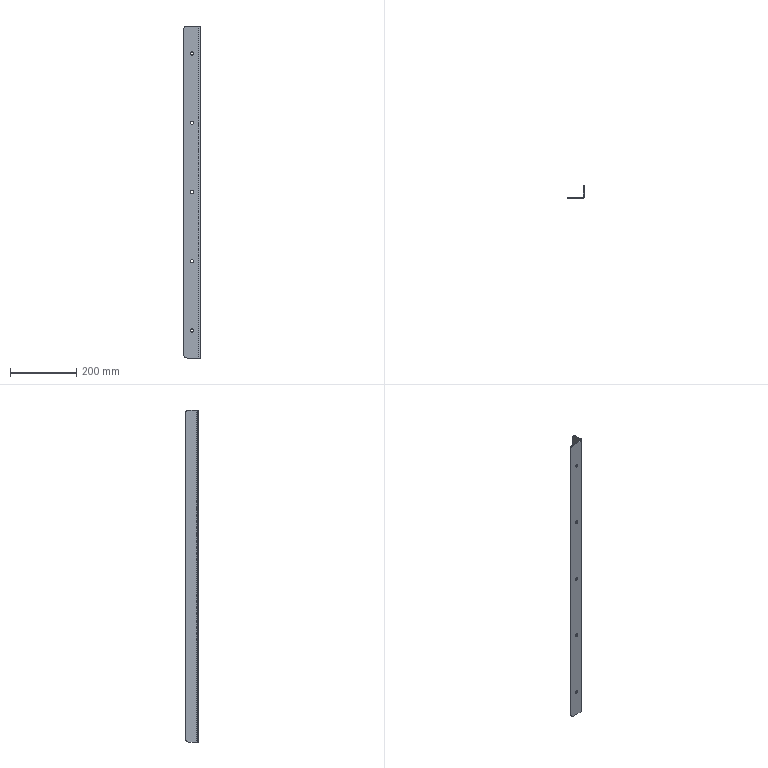Part | STEP file | 750078456 | 1 solid | 24 faces | box 50 x 40 x 1006 mm | volume 255301 mm3 | cylinder 16 | plane 8 | commonest cylinder face diameters 10 x10 20 x4 6 x1 12 x1
STEP:
#1=CARTESIAN_POINT('',(-20.,3.,210.));
#2=VERTEX_POINT('',#1);
#3=CARTESIAN_POINT('',(-30.,3.,210.));
#4=VERTEX_POINT('',#3);
#5=CARTESIAN_POINT('',(-25.,3.,210.));
#6=DIRECTION('',(0.,1.,0.));
#7=DIRECTION('',(1.,0.,0.));
#8=AXIS2_PLACEMENT_3D('',#5,#6,#7);
#9=CIRCLE('',#8,5.);
#10=EDGE_CURVE('',#2,#4,#9,.T.);
#11=ORIENTED_EDGE('',*,*,#10,.T.);
#12=CARTESIAN_POINT('',(-30.,0.,210.));
#13=VERTEX_POINT('',#12);
#14=CARTESIAN_POINT('',(-30.,1008.036,210.));
#15=DIRECTION('',(0.,-1.,0.));
#16=VECTOR('',#15,1000.);
#17=LINE('',#14,#16);
#18=EDGE_CURVE('',#4,#13,#17,.T.);
#19=ORIENTED_EDGE('',*,*,#18,.T.);
#20=CARTESIAN_POINT('',(-20.,0.,210.));
#21=VERTEX_POINT('',#20);
#22=CARTESIAN_POINT('',(-25.,0.,210.));
#23=DIRECTION('',(0.,1.,0.));
#24=DIRECTION('',(1.,0.,0.));
#25=AXIS2_PLACEMENT_3D('',#22,#23,#24);
#26=CIRCLE('',#25,5.);
#27=EDGE_CURVE('',#21,#13,#26,.T.);
#28=ORIENTED_EDGE('',*,*,#27,.F.);
#29=CARTESIAN_POINT('',(-20.,1008.036,210.));
#30=DIRECTION('',(0.,-1.,0.));
#31=VECTOR('',#30,1000.);
#32=LINE('',#29,#31);
#33=EDGE_CURVE('',#2,#21,#32,.T.);
#34=ORIENTED_EDGE('',*,*,#33,.F.);
#35=EDGE_LOOP('',(#11,#19,#28,#34));
#36=FACE_OUTER_BOUND('',#35,.T.);
#37=CARTESIAN_POINT('',(-25.,1008.036,210.));
#38=DIRECTION('',(0.,-1.,0.));
#39=DIRECTION('',(1.,0.,0.));
#40=AXIS2_PLACEMENT_3D('',#37,#38,#39);
#41=CYLINDRICAL_SURFACE('',#40,5.);
#42=ADVANCED_FACE('',(#36),#41,.F.);
#43=CARTESIAN_POINT('',(-20.,3.,-210.));
#44=VERTEX_POINT('',#43);
#45=CARTESIAN_POINT('',(-30.,3.,-210.));
#46=VERTEX_POINT('',#45);
#47=CARTESIAN_POINT('',(-25.,3.,-210.));
#48=DIRECTION('',(0.,1.,0.));
#49=DIRECTION('',(1.,0.,0.));
#50=AXIS2_PLACEMENT_3D('',#47,#48,#49);
#51=CIRCLE('',#50,5.);
#52=EDGE_CURVE('',#44,#46,#51,.T.);
#53=ORIENTED_EDGE('',*,*,#52,.T.);
#54=CARTESIAN_POINT('',(-30.,0.,-210.));
#55=VERTEX_POINT('',#54);
#56=CARTESIAN_POINT('',(-30.,1008.036,-210.));
#57=DIRECTION('',(0.,-1.,0.));
#58=VECTOR('',#57,1000.);
#59=LINE('',#56,#58);
#60=EDGE_CURVE('',#46,#55,#59,.T.);
#61=ORIENTED_EDGE('',*,*,#60,.T.);
#62=CARTESIAN_POINT('',(-20.,0.,-210.));
#63=VERTEX_POINT('',#62);
#64=CARTESIAN_POINT('',(-25.,0.,-210.));
#65=DIRECTION('',(0.,1.,0.));
#66=DIRECTION('',(1.,0.,0.));
#67=AXIS2_PLACEMENT_3D('',#64,#65,#66);
#68=CIRCLE('',#67,5.);
#69=EDGE_CURVE('',#63,#55,#68,.T.);
#70=ORIENTED_EDGE('',*,*,#69,.F.);
#71=CARTESIAN_POINT('',(-20.,1008.036,-210.));
#72=DIRECTION('',(0.,-1.,0.));
#73=VECTOR('',#72,1000.);
#74=LINE('',#71,#73);
#75=EDGE_CURVE('',#44,#63,#74,.T.);
#76=ORIENTED_EDGE('',*,*,#75,.F.);
#77=EDGE_LOOP('',(#53,#61,#70,#76));
#78=FACE_OUTER_BOUND('',#77,.T.);
#79=CARTESIAN_POINT('',(-25.,1008.036,-210.));
#80=DIRECTION('',(0.,-1.,0.));
#81=DIRECTION('',(1.,0.,0.));
#82=AXIS2_PLACEMENT_3D('',#79,#80,#81);
#83=CYLINDRICAL_SURFACE('',#82,5.);
#84=ADVANCED_FACE('',(#78),#83,.F.);
#85=CARTESIAN_POINT('',(-20.,3.,-420.));
#86=VERTEX_POINT('',#85);
#87=CARTESIAN_POINT('',(-30.,3.,-420.));
#88=VERTEX_POINT('',#87);
#89=CARTESIAN_POINT('',(-25.,3.,-420.));
#90=DIRECTION('',(0.,1.,0.));
#91=DIRECTION('',(1.,0.,0.));
#92=AXIS2_PLACEMENT_3D('',#89,#90,#91);
#93=CIRCLE('',#92,5.);
#94=EDGE_CURVE('',#86,#88,#93,.T.);
#95=ORIENTED_EDGE('',*,*,#94,.T.);
#96=CARTESIAN_POINT('',(-30.,0.,-420.));
#97=VERTEX_POINT('',#96);
#98=CARTESIAN_POINT('',(-30.,1008.036,-420.));
#99=DIRECTION('',(0.,-1.,0.));
#100=VECTOR('',#99,1000.);
#101=LINE('',#98,#100);
#102=EDGE_CURVE('',#88,#97,#101,.T.);
#103=ORIENTED_EDGE('',*,*,#102,.T.);
#104=CARTESIAN_POINT('',(-20.,0.,-420.));
#105=VERTEX_POINT('',#104);
#106=CARTESIAN_POINT('',(-25.,0.,-420.));
#107=DIRECTION('',(0.,1.,0.));
#108=DIRECTION('',(1.,0.,0.));
#109=AXIS2_PLACEMENT_3D('',#106,#107,#108);
#110=CIRCLE('',#109,5.);
#111=EDGE_CURVE('',#105,#97,#110,.T.);
#112=ORIENTED_EDGE('',*,*,#111,.F.);
#113=CARTESIAN_POINT('',(-20.,1008.036,-420.));
#114=DIRECTION('',(0.,-1.,0.));
#115=VECTOR('',#114,1000.);
#116=LINE('',#113,#115);
#117=EDGE_CURVE('',#86,#105,#116,.T.);
#118=ORIENTED_EDGE('',*,*,#117,.F.);
#119=EDGE_LOOP('',(#95,#103,#112,#118));
#120=FACE_OUTER_BOUND('',#119,.T.);
#121=CARTESIAN_POINT('',(-25.,1008.036,-420.));
#122=DIRECTION('',(0.,-1.,0.));
#123=DIRECTION('',(1.,0.,0.));
#124=AXIS2_PLACEMENT_3D('',#121,#122,#123);
#125=CYLINDRICAL_SURFACE('',#124,5.);
#126=ADVANCED_FACE('',(#120),#125,.F.);
#127=CARTESIAN_POINT('',(-20.,3.,0.));
#128=VERTEX_POINT('',#127);
#129=CARTESIAN_POINT('',(-30.,3.,0.));
#130=VERTEX_POINT('',#129);
#131=CARTESIAN_POINT('',(-25.,3.,0.));
#132=DIRECTION('',(0.,1.,0.));
#133=DIRECTION('',(1.,0.,0.));
#134=AXIS2_PLACEMENT_3D('',#131,#132,#133);
#135=CIRCLE('',#134,5.);
#136=EDGE_CURVE('',#128,#130,#135,.T.);
#137=ORIENTED_EDGE('',*,*,#136,.T.);
#138=CARTESIAN_POINT('',(-30.,0.,0.));
#139=VERTEX_POINT('',#138);
#140=CARTESIAN_POINT('',(-30.,1008.036,0.));
#141=DIRECTION('',(0.,-1.,0.));
#142=VECTOR('',#141,1000.);
#143=LINE('',#140,#142);
#144=EDGE_CURVE('',#130,#139,#143,.T.);
#145=ORIENTED_EDGE('',*,*,#144,.T.);
#146=CARTESIAN_POINT('',(-20.,0.,0.));
#147=VERTEX_POINT('',#146);
#148=CARTESIAN_POINT('',(-25.,0.,0.));
#149=DIRECTION('',(0.,1.,0.));
#150=DIRECTION('',(1.,0.,0.));
#151=AXIS2_PLACEMENT_3D('',#148,#149,#150);
#152=CIRCLE('',#151,5.);
#153=EDGE_CURVE('',#147,#139,#152,.T.);
#154=ORIENTED_EDGE('',*,*,#153,.F.);
#155=CARTESIAN_POINT('',(-20.,1008.036,0.));
#156=DIRECTION('',(0.,-1.,0.));
#157=VECTOR('',#156,1000.);
#158=LINE('',#155,#157);
#159=EDGE_CURVE('',#128,#147,#158,.T.);
#160=ORIENTED_EDGE('',*,*,#159,.F.);
#161=EDGE_LOOP('',(#137,#145,#154,#160));
#162=FACE_OUTER_BOUND('',#161,.T.);
#163=CARTESIAN_POINT('',(-25.,1008.036,0.));
#164=DIRECTION('',(0.,-1.,0.));
#165=DIRECTION('',(1.,0.,0.));
#166=AXIS2_PLACEMENT_3D('',#163,#164,#165);
#167=CYLINDRICAL_SURFACE('',#166,5.);
#168=ADVANCED_FACE('',(#162),#167,.F.);
#169=CARTESIAN_POINT('',(-20.,3.,420.));
#170=VERTEX_POINT('',#169);
#171=CARTESIAN_POINT('',(-30.,3.,420.));
#172=VERTEX_POINT('',#171);
#173=CARTESIAN_POINT('',(-25.,3.,420.));
#174=DIRECTION('',(0.,1.,0.));
#175=DIRECTION('',(1.,0.,0.));
#176=AXIS2_PLACEMENT_3D('',#173,#174,#175);
#177=CIRCLE('',#176,5.);
#178=EDGE_CURVE('',#170,#172,#177,.T.);
#179=ORIENTED_EDGE('',*,*,#178,.T.);
#180=CARTESIAN_POINT('',(-30.,0.,420.));
#181=VERTEX_POINT('',#180);
#182=CARTESIAN_POINT('',(-30.,1008.036,420.));
#183=DIRECTION('',(0.,-1.,0.));
#184=VECTOR('',#183,1000.);
#185=LINE('',#182,#184);
#186=EDGE_CURVE('',#172,#181,#185,.T.);
#187=ORIENTED_EDGE('',*,*,#186,.T.);
#188=CARTESIAN_POINT('',(-20.,0.,420.));
#189=VERTEX_POINT('',#188);
#190=CARTESIAN_POINT('',(-25.,0.,420.));
#191=DIRECTION('',(0.,1.,0.));
#192=DIRECTION('',(1.,0.,0.));
#193=AXIS2_PLACEMENT_3D('',#190,#191,#192);
#194=CIRCLE('',#193,5.);
#195=EDGE_CURVE('',#189,#181,#194,.T.);
#196=ORIENTED_EDGE('',*,*,#195,.F.);
#197=CARTESIAN_POINT('',(-20.,1008.036,420.));
#198=DIRECTION('',(0.,-1.,0.));
#199=VECTOR('',#198,1000.);
#200=LINE('',#197,#199);
#201=EDGE_CURVE('',#170,#189,#200,.T.);
#202=ORIENTED_EDGE('',*,*,#201,.F.);
#203=EDGE_LOOP('',(#179,#187,#196,#202));
#204=FACE_OUTER_BOUND('',#203,.T.);
#205=CARTESIAN_POINT('',(-25.,1008.036,420.));
#206=DIRECTION('',(0.,-1.,0.));
#207=DIRECTION('',(1.,0.,0.));
#208=AXIS2_PLACEMENT_3D('',#205,#206,#207);
#209=CYLINDRICAL_SURFACE('',#208,5.);
#210=ADVANCED_FACE('',(#204),#209,.F.);
#211=CARTESIAN_POINT('',(-40.,3.,503.));
#212=VERTEX_POINT('',#211);
#213=CARTESIAN_POINT('',(-50.,3.,493.));
#214=VERTEX_POINT('',#213);
#215=CARTESIAN_POINT('',(-40.,3.,493.));
#216=DIRECTION('',(0.,-1.,0.));
#217=DIRECTION('',(1.,0.,0.));
#218=AXIS2_PLACEMENT_3D('',#215,#216,#217);
#219=CIRCLE('',#218,10.);
#220=EDGE_CURVE('',#212,#214,#219,.T.);
#221=ORIENTED_EDGE('',*,*,#220,.F.);
#222=CARTESIAN_POINT('',(-6.,3.,503.));
#223=VERTEX_POINT('',#222);
#224=CARTESIAN_POINT('',(0.,3.,503.));
#225=DIRECTION('',(-1.,0.,0.));
#226=VECTOR('',#225,1000.);
#227=LINE('',#224,#226);
#228=EDGE_CURVE('',#223,#212,#227,.T.);
#229=ORIENTED_EDGE('',*,*,#228,.F.);
#230=CARTESIAN_POINT('',(-6.,3.,-503.));
#231=VERTEX_POINT('',#230);
#232=CARTESIAN_POINT('',(-6.,3.,503.));
#233=DIRECTION('',(0.,0.,1.));
#234=VECTOR('',#233,1000.);
#235=LINE('',#232,#234);
#236=EDGE_CURVE('',#231,#223,#235,.T.);
#237=ORIENTED_EDGE('',*,*,#236,.F.);
#238=CARTESIAN_POINT('',(-40.,3.,-503.));
#239=VERTEX_POINT('',#238);
#240=CARTESIAN_POINT('',(0.,3.,-503.));
#241=DIRECTION('',(1.,0.,0.));
#242=VECTOR('',#241,1000.);
#243=LINE('',#240,#242);
#244=EDGE_CURVE('',#239,#231,#243,.T.);
#245=ORIENTED_EDGE('',*,*,#244,.F.);
#246=CARTESIAN_POINT('',(-50.,3.,-493.));
#247=VERTEX_POINT('',#246);
#248=CARTESIAN_POINT('',(-40.,3.,-493.));
#249=DIRECTION('',(0.,-1.,0.));
#250=DIRECTION('',(-1.,0.,0.));
#251=AXIS2_PLACEMENT_3D('',#248,#249,#250);
#252=CIRCLE('',#251,10.);
#253=EDGE_CURVE('',#247,#239,#252,.T.);
#254=ORIENTED_EDGE('',*,*,#253,.F.);
#255=CARTESIAN_POINT('',(-50.,3.,503.));
#256=DIRECTION('',(0.,0.,-1.));
#257=VECTOR('',#256,1000.);
#258=LINE('',#255,#257);
#259=EDGE_CURVE('',#214,#247,#258,.T.);
#260=ORIENTED_EDGE('',*,*,#259,.F.);
#261=EDGE_LOOP('',(#221,#229,#237,#245,#254,#260));
#262=FACE_OUTER_BOUND('',#261,.T.);
#263=ORIENTED_EDGE('',*,*,#10,.F.);
#264=CARTESIAN_POINT('',(-25.,3.,210.));
#265=DIRECTION('',(0.,1.,0.));
#266=DIRECTION('',(1.,0.,0.));
#267=AXIS2_PLACEMENT_3D('',#264,#265,#266);
#268=CIRCLE('',#267,5.);
#269=EDGE_CURVE('',#4,#2,#268,.T.);
#270=ORIENTED_EDGE('',*,*,#269,.F.);
#271=EDGE_LOOP('',(#263,#270));
#272=FACE_BOUND('',#271,.T.);
#273=ORIENTED_EDGE('',*,*,#52,.F.);
#274=CARTESIAN_POINT('',(-25.,3.,-210.));
#275=DIRECTION('',(0.,1.,0.));
#276=DIRECTION('',(1.,0.,0.));
#277=AXIS2_PLACEMENT_3D('',#274,#275,#276);
#278=CIRCLE('',#277,5.);
#279=EDGE_CURVE('',#46,#44,#278,.T.);
#280=ORIENTED_EDGE('',*,*,#279,.F.);
#281=EDGE_LOOP('',(#273,#280));
#282=FACE_BOUND('',#281,.T.);
#283=ORIENTED_EDGE('',*,*,#94,.F.);
#284=CARTESIAN_POINT('',(-25.,3.,-420.));
#285=DIRECTION('',(0.,1.,0.));
#286=DIRECTION('',(1.,0.,0.));
#287=AXIS2_PLACEMENT_3D('',#284,#285,#286);
#288=CIRCLE('',#287,5.);
#289=EDGE_CURVE('',#88,#86,#288,.T.);
#290=ORIENTED_EDGE('',*,*,#289,.F.);
#291=EDGE_LOOP('',(#283,#290));
#292=FACE_BOUND('',#291,.T.);
#293=ORIENTED_EDGE('',*,*,#136,.F.);
#294=CARTESIAN_POINT('',(-25.,3.,0.));
#295=DIRECTION('',(0.,1.,0.));
#296=DIRECTION('',(1.,0.,0.));
#297=AXIS2_PLACEMENT_3D('',#294,#295,#296);
#298=CIRCLE('',#297,5.);
#299=EDGE_CURVE('',#130,#128,#298,.T.);
#300=ORIENTED_EDGE('',*,*,#299,.F.);
#301=EDGE_LOOP('',(#293,#300));
#302=FACE_BOUND('',#301,.T.);
#303=ORIENTED_EDGE('',*,*,#178,.F.);
#304=CARTESIAN_POINT('',(-25.,3.,420.));
#305=DIRECTION('',(0.,1.,0.));
#306=DIRECTION('',(1.,0.,0.));
#307=AXIS2_PLACEMENT_3D('',#304,#305,#306);
#308=CIRCLE('',#307,5.);
#309=EDGE_CURVE('',#172,#170,#308,.T.);
#310=ORIENTED_EDGE('',*,*,#309,.F.);
#311=EDGE_LOOP('',(#303,#310));
#312=FACE_BOUND('',#311,.T.);
#313=CARTESIAN_POINT('',(0.,3.,503.));
#314=DIRECTION('',(0.,-1.,0.));
#315=DIRECTION('',(1.,0.,0.));
#316=AXIS2_PLACEMENT_3D('',#313,#314,#315);
#317=PLANE('',#316);
#318=ADVANCED_FACE('',(#262,#272,#282,#292,#302,#312),#317,.F.);
#319=ORIENTED_EDGE('',*,*,#259,.T.);
#320=CARTESIAN_POINT('',(-50.,0.,-493.));
#321=VERTEX_POINT('',#320);
#322=CARTESIAN_POINT('',(-50.,0.,-493.));
#323=DIRECTION('',(0.,-1.,0.));
#324=VECTOR('',#323,1000.);
#325=LINE('',#322,#324);
#326=EDGE_CURVE('',#247,#321,#325,.T.);
#327=ORIENTED_EDGE('',*,*,#326,.T.);
#328=CARTESIAN_POINT('',(-50.,0.,493.));
#329=VERTEX_POINT('',#328);
#330=CARTESIAN_POINT('',(-50.,0.,503.));
#331=DIRECTION('',(0.,0.,1.));
#332=VECTOR('',#331,1000.);
#333=LINE('',#330,#332);
#334=EDGE_CURVE('',#321,#329,#333,.T.);
#335=ORIENTED_EDGE('',*,*,#334,.T.);
#336=CARTESIAN_POINT('',(-50.,0.,493.));
#337=DIRECTION('',(0.,1.,0.));
#338=VECTOR('',#337,1000.);
#339=LINE('',#336,#338);
#340=EDGE_CURVE('',#329,#214,#339,.T.);
#341=ORIENTED_EDGE('',*,*,#340,.T.);
#342=EDGE_LOOP('',(#319,#327,#335,#341));
#343=FACE_OUTER_BOUND('',#342,.T.);
#344=CARTESIAN_POINT('',(-50.,0.,503.));
#345=DIRECTION('',(-1.,0.,0.));
#346=DIRECTION('',(0.,-1.,0.));
#347=AXIS2_PLACEMENT_3D('',#344,#345,#346);
#348=PLANE('',#347);
#349=ADVANCED_FACE('',(#343),#348,.T.);
#350=CARTESIAN_POINT('',(-40.,0.,503.));
#351=VERTEX_POINT('',#350);
#352=CARTESIAN_POINT('',(-40.,0.,493.));
#353=DIRECTION('',(0.,1.,0.));
#354=DIRECTION('',(1.,0.,0.));
#355=AXIS2_PLACEMENT_3D('',#352,#353,#354);
#356=CIRCLE('',#355,10.);
#357=EDGE_CURVE('',#329,#351,#356,.T.);
#358=ORIENTED_EDGE('',*,*,#357,.T.);
#359=CARTESIAN_POINT('',(-40.,0.,503.));
#360=DIRECTION('',(0.,1.,0.));
#361=VECTOR('',#360,1000.);
#362=LINE('',#359,#361);
#363=EDGE_CURVE('',#351,#212,#362,.T.);
#364=ORIENTED_EDGE('',*,*,#363,.T.);
#365=ORIENTED_EDGE('',*,*,#220,.T.);
#366=ORIENTED_EDGE('',*,*,#340,.F.);
#367=EDGE_LOOP('',(#358,#364,#365,#366));
#368=FACE_OUTER_BOUND('',#367,.T.);
#369=CARTESIAN_POINT('',(-40.,0.,493.));
#370=DIRECTION('',(0.,-1.,0.));
#371=DIRECTION('',(1.,0.,0.));
#372=AXIS2_PLACEMENT_3D('',#369,#370,#371);
#373=CYLINDRICAL_SURFACE('',#372,10.);
#374=ADVANCED_FACE('',(#368),#373,.T.);
#375=CARTESIAN_POINT('',(-6.,0.,503.));
#376=VERTEX_POINT('',#375);
#377=CARTESIAN_POINT('',(0.,0.,503.));
#378=DIRECTION('',(1.,0.,0.));
#379=VECTOR('',#378,1000.);
#380=LINE('',#377,#379);
#381=EDGE_CURVE('',#351,#376,#380,.T.);
#382=ORIENTED_EDGE('',*,*,#381,.T.);
#383=CARTESIAN_POINT('',(0.,6.,503.));
#384=VERTEX_POINT('',#383);
#385=CARTESIAN_POINT('',(-6.,6.,503.));
#386=DIRECTION('',(0.,0.,1.));
#387=DIRECTION('',(-1.,0.,0.));
#388=AXIS2_PLACEMENT_3D('',#385,#386,#387);
#389=CIRCLE('',#388,6.);
#390=EDGE_CURVE('',#376,#384,#389,.T.);
#391=ORIENTED_EDGE('',*,*,#390,.T.);
#392=CARTESIAN_POINT('',(0.,30.,503.));
#393=VERTEX_POINT('',#392);
#394=CARTESIAN_POINT('',(0.,0.,503.));
#395=DIRECTION('',(0.,1.,0.));
#396=VECTOR('',#395,1000.);
#397=LINE('',#394,#396);
#398=EDGE_CURVE('',#384,#393,#397,.T.);
#399=ORIENTED_EDGE('',*,*,#398,.T.);
#400=CARTESIAN_POINT('',(-3.,30.,503.));
#401=VERTEX_POINT('',#400);
#402=CARTESIAN_POINT('',(0.,30.,503.));
#403=DIRECTION('',(-1.,0.,0.));
#404=VECTOR('',#403,1000.);
#405=LINE('',#402,#404);
#406=EDGE_CURVE('',#393,#401,#405,.T.);
#407=ORIENTED_EDGE('',*,*,#406,.T.);
#408=CARTESIAN_POINT('',(-3.,6.,503.));
#409=VERTEX_POINT('',#408);
#410=CARTESIAN_POINT('',(-3.,0.,503.));
#411=DIRECTION('',(0.,-1.,0.));
#412=VECTOR('',#411,1000.);
#413=LINE('',#410,#412);
#414=EDGE_CURVE('',#401,#409,#413,.T.);
#415=ORIENTED_EDGE('',*,*,#414,.T.);
#416=CARTESIAN_POINT('',(-6.,6.,503.));
#417=DIRECTION('',(0.,0.,-1.));
#418=DIRECTION('',(-1.,0.,0.));
#419=AXIS2_PLACEMENT_3D('',#416,#417,#418);
#420=CIRCLE('',#419,3.);
#421=EDGE_CURVE('',#409,#223,#420,.T.);
#422=ORIENTED_EDGE('',*,*,#421,.T.);
#423=ORIENTED_EDGE('',*,*,#228,.T.);
#424=ORIENTED_EDGE('',*,*,#363,.F.);
#425=EDGE_LOOP('',(#382,#391,#399,#407,#415,#422,#423,#424));
#426=FACE_OUTER_BOUND('',#425,.T.);
#427=CARTESIAN_POINT('',(0.,0.,503.));
#428=DIRECTION('',(0.,0.,1.));
#429=DIRECTION('',(1.,0.,0.));
#430=AXIS2_PLACEMENT_3D('',#427,#428,#429);
#431=PLANE('',#430);
#432=ADVANCED_FACE('',(#426),#431,.T.);
#433=ORIENTED_EDGE('',*,*,#236,.T.);
#434=ORIENTED_EDGE('',*,*,#421,.F.);
#435=CARTESIAN_POINT('',(-3.,6.,-503.));
#436=VERTEX_POINT('',#435);
#437=CARTESIAN_POINT('',(-3.,6.,503.));
#438=DIRECTION('',(0.,0.,1.));
#439=VECTOR('',#438,1000.);
#440=LINE('',#437,#439);
#441=EDGE_CURVE('',#436,#409,#440,.T.);
#442=ORIENTED_EDGE('',*,*,#441,.F.);
#443=CARTESIAN_POINT('',(-6.,6.,-503.));
#444=DIRECTION('',(0.,0.,1.));
#445=DIRECTION('',(-1.,0.,0.));
#446=AXIS2_PLACEMENT_3D('',#443,#444,#445);
#447=CIRCLE('',#446,3.);
#448=EDGE_CURVE('',#231,#436,#447,.T.);
#449=ORIENTED_EDGE('',*,*,#448,.F.);
#450=EDGE_LOOP('',(#433,#434,#442,#449));
#451=FACE_OUTER_BOUND('',#450,.T.);
#452=CARTESIAN_POINT('',(-6.,6.,503.));
#453=DIRECTION('',(0.,0.,-1.));
#454=DIRECTION('',(-1.,0.,0.));
#455=AXIS2_PLACEMENT_3D('',#452,#453,#454);
#456=CYLINDRICAL_SURFACE('',#455,3.);
#457=ADVANCED_FACE('',(#451),#456,.F.);
#458=CARTESIAN_POINT('',(-40.,0.,-503.));
#459=VERTEX_POINT('',#458);
#460=CARTESIAN_POINT('',(-40.,40.,-503.));
#461=DIRECTION('',(0.,-1.,0.));
#462=VECTOR('',#461,1000.);
#463=LINE('',#460,#462);
#464=EDGE_CURVE('',#239,#459,#463,.T.);
#465=ORIENTED_EDGE('',*,*,#464,.F.);
#466=ORIENTED_EDGE('',*,*,#244,.T.);
#467=ORIENTED_EDGE('',*,*,#448,.T.);
#468=CARTESIAN_POINT('',(-3.,30.,-503.));
#469=VERTEX_POINT('',#468);
#470=CARTESIAN_POINT('',(-3.,40.,-503.));
#471=DIRECTION('',(0.,-1.,0.));
#472=VECTOR('',#471,1000.);
#473=LINE('',#470,#472);
#474=EDGE_CURVE('',#469,#436,#473,.T.);
#475=ORIENTED_EDGE('',*,*,#474,.F.);
#476=CARTESIAN_POINT('',(0.,30.,-503.));
#477=VERTEX_POINT('',#476);
#478=CARTESIAN_POINT('',(0.,30.,-503.));
#479=DIRECTION('',(-1.,0.,0.));
#480=VECTOR('',#479,1000.);
#481=LINE('',#478,#480);
#482=EDGE_CURVE('',#477,#469,#481,.T.);
#483=ORIENTED_EDGE('',*,*,#482,.F.);
#484=CARTESIAN_POINT('',(0.,6.,-503.));
#485=VERTEX_POINT('',#484);
#486=CARTESIAN_POINT('',(0.,40.,-503.));
#487=DIRECTION('',(0.,1.,0.));
#488=VECTOR('',#487,1000.);
#489=LINE('',#486,#488);
#490=EDGE_CURVE('',#485,#477,#489,.T.);
#491=ORIENTED_EDGE('',*,*,#490,.F.);
#492=CARTESIAN_POINT('',(-6.,0.,-503.));
#493=VERTEX_POINT('',#492);
#494=CARTESIAN_POINT('',(-6.,6.,-503.));
#495=DIRECTION('',(0.,0.,1.));
#496=DIRECTION('',(-1.,0.,0.));
#497=AXIS2_PLACEMENT_3D('',#494,#495,#496);
#498=CIRCLE('',#497,6.);
#499=EDGE_CURVE('',#493,#485,#498,.T.);
#500=ORIENTED_EDGE('',*,*,#499,.F.);
#501=CARTESIAN_POINT('',(0.,0.,-503.));
#502=DIRECTION('',(1.,0.,0.));
#503=VECTOR('',#502,1000.);
#504=LINE('',#501,#503);
#505=EDGE_CURVE('',#459,#493,#504,.T.);
#506=ORIENTED_EDGE('',*,*,#505,.F.);
#507=EDGE_LOOP('',(#465,#466,#467,#475,#483,#491,#500,#506));
#508=FACE_OUTER_BOUND('',#507,.T.);
#509=CARTESIAN_POINT('',(0.,40.,-503.));
#510=DIRECTION('',(0.,0.,1.));
#511=DIRECTION('',(1.,0.,0.));
#512=AXIS2_PLACEMENT_3D('',#509,#510,#511);
#513=PLANE('',#512);
#514=ADVANCED_FACE('',(#508),#513,.F.);
#515=CARTESIAN_POINT('',(-40.,0.,-493.));
#516=DIRECTION('',(0.,1.,0.));
#517=DIRECTION('',(-1.,0.,0.));
#518=AXIS2_PLACEMENT_3D('',#515,#516,#517);
#519=CIRCLE('',#518,10.);
#520=EDGE_CURVE('',#459,#321,#519,.T.);
#521=ORIENTED_EDGE('',*,*,#520,.T.);
#522=ORIENTED_EDGE('',*,*,#326,.F.);
#523=ORIENTED_EDGE('',*,*,#253,.T.);
#524=ORIENTED_EDGE('',*,*,#464,.T.);
#525=EDGE_LOOP('',(#521,#522,#523,#524));
#526=FACE_OUTER_BOUND('',#525,.T.);
#527=CARTESIAN_POINT('',(-40.,0.,-493.));
#528=DIRECTION('',(0.,1.,0.));
#529=DIRECTION('',(-1.,0.,0.));
#530=AXIS2_PLACEMENT_3D('',#527,#528,#529);
#531=CYLINDRICAL_SURFACE('',#530,10.);
#532=ADVANCED_FACE('',(#526),#531,.T.);
#533=ORIENTED_EDGE('',*,*,#18,.F.);
#534=ORIENTED_EDGE('',*,*,#269,.T.);
#535=ORIENTED_EDGE('',*,*,#33,.T.);
#536=CARTESIAN_POINT('',(-25.,0.,210.));
#537=DIRECTION('',(0.,1.,0.));
#538=DIRECTION('',(1.,0.,0.));
#539=AXIS2_PLACEMENT_3D('',#536,#537,#538);
#540=CIRCLE('',#539,5.);
#541=EDGE_CURVE('',#13,#21,#540,.T.);
#542=ORIENTED_EDGE('',*,*,#541,.F.);
#543=EDGE_LOOP('',(#533,#534,#535,#542));
#544=FACE_OUTER_BOUND('',#543,.T.);
#545=CARTESIAN_POINT('',(-25.,1008.036,210.));
#546=DIRECTION('',(0.,-1.,0.));
#547=DIRECTION('',(1.,0.,0.));
#548=AXIS2_PLACEMENT_3D('',#545,#546,#547);
#549=CYLINDRICAL_SURFACE('',#548,5.);
#550=ADVANCED_FACE('',(#544),#549,.F.);
#551=ORIENTED_EDGE('',*,*,#60,.F.);
#552=ORIENTED_EDGE('',*,*,#279,.T.);
#553=ORIENTED_EDGE('',*,*,#75,.T.);
#554=CARTESIAN_POINT('',(-25.,0.,-210.));
#555=DIRECTION('',(0.,1.,0.));
#556=DIRECTION('',(1.,0.,0.));
#557=AXIS2_PLACEMENT_3D('',#554,#555,#556);
#558=CIRCLE('',#557,5.);
#559=EDGE_CURVE('',#55,#63,#558,.T.);
#560=ORIENTED_EDGE('',*,*,#559,.F.);
#561=EDGE_LOOP('',(#551,#552,#553,#560));
#562=FACE_OUTER_BOUND('',#561,.T.);
#563=CARTESIAN_POINT('',(-25.,1008.036,-210.));
#564=DIRECTION('',(0.,-1.,0.));
#565=DIRECTION('',(1.,0.,0.));
#566=AXIS2_PLACEMENT_3D('',#563,#564,#565);
#567=CYLINDRICAL_SURFACE('',#566,5.);
#568=ADVANCED_FACE('',(#562),#567,.F.);
#569=ORIENTED_EDGE('',*,*,#102,.F.);
#570=ORIENTED_EDGE('',*,*,#289,.T.);
#571=ORIENTED_EDGE('',*,*,#117,.T.);
#572=CARTESIAN_POINT('',(-25.,0.,-420.));
#573=DIRECTION('',(0.,1.,0.));
#574=DIRECTION('',(1.,0.,0.));
#575=AXIS2_PLACEMENT_3D('',#572,#573,#574);
#576=CIRCLE('',#575,5.);
#577=EDGE_CURVE('',#97,#105,#576,.T.);
#578=ORIENTED_EDGE('',*,*,#577,.F.);
#579=EDGE_LOOP('',(#569,#570,#571,#578));
#580=FACE_OUTER_BOUND('',#579,.T.);
#581=CARTESIAN_POINT('',(-25.,1008.036,-420.));
#582=DIRECTION('',(0.,-1.,0.));
#583=DIRECTION('',(1.,0.,0.));
#584=AXIS2_PLACEMENT_3D('',#581,#582,#583);
#585=CYLINDRICAL_SURFACE('',#584,5.);
#586=ADVANCED_FACE('',(#580),#585,.F.);
#587=ORIENTED_EDGE('',*,*,#144,.F.);
#588=ORIENTED_EDGE('',*,*,#299,.T.);
#589=ORIENTED_EDGE('',*,*,#159,.T.);
#590=CARTESIAN_POINT('',(-25.,0.,0.));
#591=DIRECTION('',(0.,1.,0.));
#592=DIRECTION('',(1.,0.,0.));
#593=AXIS2_PLACEMENT_3D('',#590,#591,#592);
#594=CIRCLE('',#593,5.);
#595=EDGE_CURVE('',#139,#147,#594,.T.);
#596=ORIENTED_EDGE('',*,*,#595,.F.);
#597=EDGE_LOOP('',(#587,#588,#589,#596));
#598=FACE_OUTER_BOUND('',#597,.T.);
#599=CARTESIAN_POINT('',(-25.,1008.036,0.));
#600=DIRECTION('',(0.,-1.,0.));
#601=DIRECTION('',(1.,0.,0.));
#602=AXIS2_PLACEMENT_3D('',#599,#600,#601);
#603=CYLINDRICAL_SURFACE('',#602,5.);
#604=ADVANCED_FACE('',(#598),#603,.F.);
#605=ORIENTED_EDGE('',*,*,#186,.F.);
#606=ORIENTED_EDGE('',*,*,#309,.T.);
#607=ORIENTED_EDGE('',*,*,#201,.T.);
#608=CARTESIAN_POINT('',(-25.,0.,420.));
#609=DIRECTION('',(0.,1.,0.));
#610=DIRECTION('',(1.,0.,0.));
#611=AXIS2_PLACEMENT_3D('',#608,#609,#610);
#612=CIRCLE('',#611,5.);
#613=EDGE_CURVE('',#181,#189,#612,.T.);
#614=ORIENTED_EDGE('',*,*,#613,.F.);
#615=EDGE_LOOP('',(#605,#606,#607,#614));
#616=FACE_OUTER_BOUND('',#615,.T.);
#617=CARTESIAN_POINT('',(-25.,1008.036,420.));
#618=DIRECTION('',(0.,-1.,0.));
#619=DIRECTION('',(1.,0.,0.));
#620=AXIS2_PLACEMENT_3D('',#617,#618,#619);
#621=CYLINDRICAL_SURFACE('',#620,5.);
#622=ADVANCED_FACE('',(#616),#621,.F.);
#623=ORIENTED_EDGE('',*,*,#505,.T.);
#624=CARTESIAN_POINT('',(-6.,0.,503.));
#625=DIRECTION('',(0.,0.,1.));
#626=VECTOR('',#625,1000.);
#627=LINE('',#624,#626);
#628=EDGE_CURVE('',#493,#376,#627,.T.);
#629=ORIENTED_EDGE('',*,*,#628,.T.);
#630=ORIENTED_EDGE('',*,*,#381,.F.);
#631=ORIENTED_EDGE('',*,*,#357,.F.);
#632=ORIENTED_EDGE('',*,*,#334,.F.);
#633=ORIENTED_EDGE('',*,*,#520,.F.);
#634=EDGE_LOOP('',(#623,#629,#630,#631,#632,#633));
#635=FACE_OUTER_BOUND('',#634,.T.);
#636=ORIENTED_EDGE('',*,*,#27,.T.);
#637=ORIENTED_EDGE('',*,*,#541,.T.);
#638=EDGE_LOOP('',(#636,#637));
#639=FACE_BOUND('',#638,.T.);
#640=ORIENTED_EDGE('',*,*,#69,.T.);
#641=ORIENTED_EDGE('',*,*,#559,.T.);
#642=EDGE_LOOP('',(#640,#641));
#643=FACE_BOUND('',#642,.T.);
#644=ORIENTED_EDGE('',*,*,#111,.T.);
#645=ORIENTED_EDGE('',*,*,#577,.T.);
#646=EDGE_LOOP('',(#644,#645));
#647=FACE_BOUND('',#646,.T.);
#648=ORIENTED_EDGE('',*,*,#153,.T.);
#649=ORIENTED_EDGE('',*,*,#595,.T.);
#650=EDGE_LOOP('',(#648,#649));
#651=FACE_BOUND('',#650,.T.);
#652=ORIENTED_EDGE('',*,*,#195,.T.);
#653=ORIENTED_EDGE('',*,*,#613,.T.);
#654=EDGE_LOOP('',(#652,#653));
#655=FACE_BOUND('',#654,.T.);
#656=CARTESIAN_POINT('',(0.,0.,503.));
#657=DIRECTION('',(0.,-1.,0.));
#658=DIRECTION('',(1.,0.,0.));
#659=AXIS2_PLACEMENT_3D('',#656,#657,#658);
#660=PLANE('',#659);
#661=ADVANCED_FACE('',(#635,#639,#643,#647,#651,#655),#660,.T.);
#662=ORIENTED_EDGE('',*,*,#390,.F.);
#663=ORIENTED_EDGE('',*,*,#628,.F.);
#664=ORIENTED_EDGE('',*,*,#499,.T.);
#665=CARTESIAN_POINT('',(0.,6.,503.));
#666=DIRECTION('',(0.,0.,1.));
#667=VECTOR('',#666,1000.);
#668=LINE('',#665,#667);
#669=EDGE_CURVE('',#485,#384,#668,.T.);
#670=ORIENTED_EDGE('',*,*,#669,.T.);
#671=EDGE_LOOP('',(#662,#663,#664,#670));
#672=FACE_OUTER_BOUND('',#671,.T.);
#673=CARTESIAN_POINT('',(-6.,6.,503.));
#674=DIRECTION('',(0.,0.,-1.));
#675=DIRECTION('',(-1.,0.,0.));
#676=AXIS2_PLACEMENT_3D('',#673,#674,#675);
#677=CYLINDRICAL_SURFACE('',#676,6.);
#678=ADVANCED_FACE('',(#672),#677,.T.);
#679=CARTESIAN_POINT('',(-3.,40.,493.));
#680=VERTEX_POINT('',#679);
#681=CARTESIAN_POINT('',(-3.,30.,493.));
#682=DIRECTION('',(1.,0.,0.));
#683=DIRECTION('',(0.,0.,1.));
#684=AXIS2_PLACEMENT_3D('',#681,#682,#683);
#685=CIRCLE('',#684,10.);
#686=EDGE_CURVE('',#680,#401,#685,.T.);
#687=ORIENTED_EDGE('',*,*,#686,.F.);
#688=CARTESIAN_POINT('',(-3.,40.,-493.));
#689=VERTEX_POINT('',#688);
#690=CARTESIAN_POINT('',(-3.,40.,503.));
#691=DIRECTION('',(0.,0.,1.));
#692=VECTOR('',#691,1000.);
#693=LINE('',#690,#692);
#694=EDGE_CURVE('',#689,#680,#693,.T.);
#695=ORIENTED_EDGE('',*,*,#694,.F.);
#696=CARTESIAN_POINT('',(-3.,30.,-493.));
#697=DIRECTION('',(1.,0.,0.));
#698=DIRECTION('',(0.,0.,-1.));
#699=AXIS2_PLACEMENT_3D('',#696,#697,#698);
#700=CIRCLE('',#699,10.);
#701=EDGE_CURVE('',#469,#689,#700,.T.);
#702=ORIENTED_EDGE('',*,*,#701,.F.);
#703=ORIENTED_EDGE('',*,*,#474,.T.);
#704=ORIENTED_EDGE('',*,*,#441,.T.);
#705=ORIENTED_EDGE('',*,*,#414,.F.);
#706=EDGE_LOOP('',(#687,#695,#702,#703,#704,#705));
#707=FACE_OUTER_BOUND('',#706,.T.);
#708=CARTESIAN_POINT('',(-3.,40.,503.));
#709=DIRECTION('',(1.,0.,0.));
#710=DIRECTION('',(0.,0.,-1.));
#711=AXIS2_PLACEMENT_3D('',#708,#709,#710);
#712=PLANE('',#711);
#713=ADVANCED_FACE('',(#707),#712,.F.);
#714=CARTESIAN_POINT('',(0.,40.,493.));
#715=VERTEX_POINT('',#714);
#716=CARTESIAN_POINT('',(0.,30.,493.));
#717=DIRECTION('',(-1.,0.,0.));
#718=DIRECTION('',(0.,0.,1.));
#719=AXIS2_PLACEMENT_3D('',#716,#717,#718);
#720=CIRCLE('',#719,10.);
#721=EDGE_CURVE('',#393,#715,#720,.T.);
#722=ORIENTED_EDGE('',*,*,#721,.T.);
#723=CARTESIAN_POINT('',(0.,40.,493.));
#724=DIRECTION('',(-1.,0.,0.));
#725=VECTOR('',#724,1000.);
#726=LINE('',#723,#725);
#727=EDGE_CURVE('',#715,#680,#726,.T.);
#728=ORIENTED_EDGE('',*,*,#727,.T.);
#729=ORIENTED_EDGE('',*,*,#686,.T.);
#730=ORIENTED_EDGE('',*,*,#406,.F.);
#731=EDGE_LOOP('',(#722,#728,#729,#730));
#732=FACE_OUTER_BOUND('',#731,.T.);
#733=CARTESIAN_POINT('',(0.,30.,493.));
#734=DIRECTION('',(-1.,0.,0.));
#735=DIRECTION('',(0.,0.,1.));
#736=AXIS2_PLACEMENT_3D('',#733,#734,#735);
#737=CYLINDRICAL_SURFACE('',#736,10.);
#738=ADVANCED_FACE('',(#732),#737,.T.);
#739=ORIENTED_EDGE('',*,*,#490,.T.);
#740=CARTESIAN_POINT('',(0.,40.,-493.));
#741=VERTEX_POINT('',#740);
#742=CARTESIAN_POINT('',(0.,30.,-493.));
#743=DIRECTION('',(1.,0.,0.));
#744=DIRECTION('',(0.,0.,-1.));
#745=AXIS2_PLACEMENT_3D('',#742,#743,#744);
#746=CIRCLE('',#745,10.);
#747=EDGE_CURVE('',#477,#741,#746,.T.);
#748=ORIENTED_EDGE('',*,*,#747,.T.);
#749=CARTESIAN_POINT('',(0.,40.,503.));
#750=DIRECTION('',(0.,0.,1.));
#751=VECTOR('',#750,1000.);
#752=LINE('',#749,#751);
#753=EDGE_CURVE('',#741,#715,#752,.T.);
#754=ORIENTED_EDGE('',*,*,#753,.T.);
#755=ORIENTED_EDGE('',*,*,#721,.F.);
#756=ORIENTED_EDGE('',*,*,#398,.F.);
#757=ORIENTED_EDGE('',*,*,#669,.F.);
#758=EDGE_LOOP('',(#739,#748,#754,#755,#756,#757));
#759=FACE_OUTER_BOUND('',#758,.T.);
#760=CARTESIAN_POINT('',(0.,40.,503.));
#761=DIRECTION('',(1.,0.,0.));
#762=DIRECTION('',(0.,0.,-1.));
#763=AXIS2_PLACEMENT_3D('',#760,#761,#762);
#764=PLANE('',#763);
#765=ADVANCED_FACE('',(#759),#764,.T.);
#766=ORIENTED_EDGE('',*,*,#747,.F.);
#767=ORIENTED_EDGE('',*,*,#482,.T.);
#768=ORIENTED_EDGE('',*,*,#701,.T.);
#769=CARTESIAN_POINT('',(0.,40.,-493.));
#770=DIRECTION('',(1.,0.,0.));
#771=VECTOR('',#770,1000.);
#772=LINE('',#769,#771);
#773=EDGE_CURVE('',#689,#741,#772,.T.);
#774=ORIENTED_EDGE('',*,*,#773,.T.);
#775=EDGE_LOOP('',(#766,#767,#768,#774));
#776=FACE_OUTER_BOUND('',#775,.T.);
#777=CARTESIAN_POINT('',(0.,30.,-493.));
#778=DIRECTION('',(1.,0.,0.));
#779=DIRECTION('',(0.,0.,-1.));
#780=AXIS2_PLACEMENT_3D('',#777,#778,#779);
#781=CYLINDRICAL_SURFACE('',#780,10.);
#782=ADVANCED_FACE('',(#776),#781,.T.);
#783=ORIENTED_EDGE('',*,*,#727,.F.);
#784=ORIENTED_EDGE('',*,*,#753,.F.);
#785=ORIENTED_EDGE('',*,*,#773,.F.);
#786=ORIENTED_EDGE('',*,*,#694,.T.);
#787=EDGE_LOOP('',(#783,#784,#785,#786));
#788=FACE_OUTER_BOUND('',#787,.T.);
#789=CARTESIAN_POINT('',(0.,40.,503.));
#790=DIRECTION('',(0.,-1.,0.));
#791=DIRECTION('',(0.,0.,-1.));
#792=AXIS2_PLACEMENT_3D('',#789,#790,#791);
#793=PLANE('',#792);
#794=ADVANCED_FACE('',(#788),#793,.F.);
#795=CLOSED_SHELL('',(#42,#84,#126,#168,#210,#318,#349,#374,#432,#457,#514,#532,#550,#568,#586,#604,#622,#661,#678,#713,#738,#765,#782,#794));
#796=MANIFOLD_SOLID_BREP('',#795);
#797=CARTESIAN_POINT('',(0.,0.,0.));
#798=DIRECTION('',(0.,0.,1.));
#799=DIRECTION('',(1.,0.,0.));
#800=AXIS2_PLACEMENT_3D('',#797,#798,#799);
#801=(LENGTH_UNIT()NAMED_UNIT(*)SI_UNIT(.MILLI.,.METRE.));
#802=UNCERTAINTY_MEASURE_WITH_UNIT(LENGTH_MEASURE(0.00001),#801,'','');
#803=(NAMED_UNIT(*)PLANE_ANGLE_UNIT()SI_UNIT($,.RADIAN.));
#804=(NAMED_UNIT(*)SI_UNIT($,.STERADIAN.)SOLID_ANGLE_UNIT());
#805=(GEOMETRIC_REPRESENTATION_CONTEXT(3)GLOBAL_UNCERTAINTY_ASSIGNED_CONTEXT((#802))GLOBAL_UNIT_ASSIGNED_CONTEXT((#801,#803,#804))REPRESENTATION_CONTEXT('',''));
#806=ADVANCED_BREP_SHAPE_REPRESENTATION('',(#796,#800),#805);